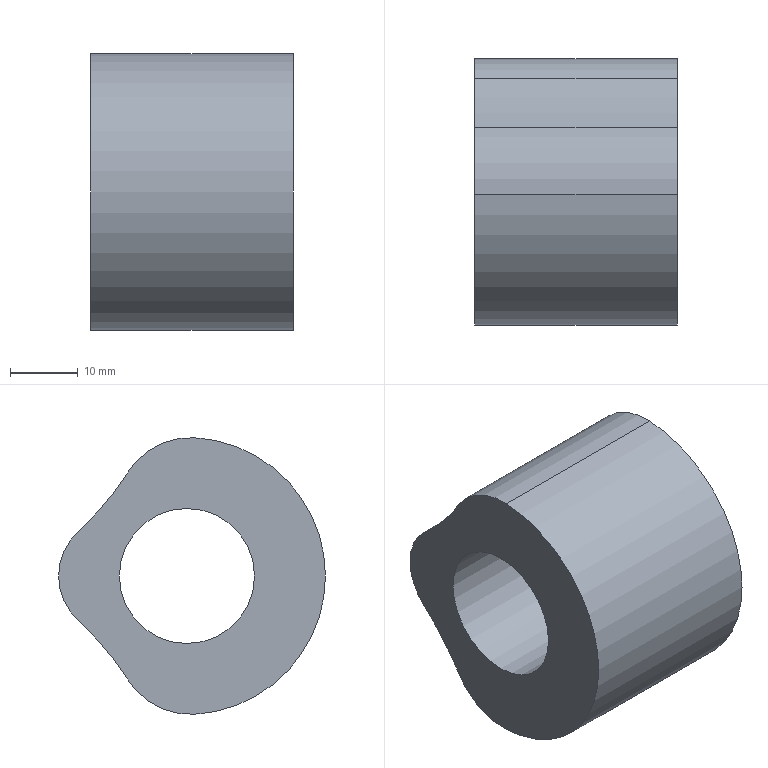Part | STEP file | cuozhitulun | 1 solid | 9 faces | box 30 x 39.5 x 40.969 mm | volume 25744 mm3 | cylinder 7 | plane 2 | commonest cylinder face diameters 22 x2 76 x2 18 x1 20 x1 41 x1
STEP:
#1=CARTESIAN_POINT('',(0.,0.,0.));
#2=DIRECTION('',(0.,0.,1.));
#3=DIRECTION('',(1.,0.,0.));
#4=AXIS2_PLACEMENT_3D('',#1,#2,#3);
#5=CARTESIAN_POINT('',(15.,8.833,-15.245));
#6=VERTEX_POINT('',#5);
#7=CARTESIAN_POINT('',(15.,15.975,-6.73));
#8=VERTEX_POINT('',#7);
#9=CARTESIAN_POINT('',(15.,41.205,-35.146));
#10=DIRECTION('',(-1.,0.,0.));
#11=DIRECTION('',(0.,0.,-1.));
#12=AXIS2_PLACEMENT_3D('',#9,#10,#11);
#13=CIRCLE('',#12,38.);
#14=CARTESIAN_POINT('',(15.,20.333,-22.315));
#15=DIRECTION('',(1.,0.,0.));
#16=DIRECTION('',(0.,0.,-1.));
#17=AXIS2_PLACEMENT_3D('',#14,#15,#16);
#18=PLANE('',#17);
#19=CARTESIAN_POINT('',(50.831,20.872));
#20=CARTESIAN_POINT('',(50.831,-44.946));
#21=CARTESIAN_POINT('',(-6.169,-12.037));
#22=CARTESIAN_POINT('',(-63.169,20.872));
#23=CARTESIAN_POINT('',(-6.169,53.781));
#24=CARTESIAN_POINT('',(50.831,86.69));
#25=CARTESIAN_POINT('',(50.831,20.872));
#26=(BOUNDED_CURVE()B_SPLINE_CURVE(2,(#19,#20,#21,#22,#23,#24,#25),.UNSPECIFIED.,.T.,.F.)B_SPLINE_CURVE_WITH_KNOTS((1,2,2,2,2,1),(-2.094,0.,2.094,4.189,6.283,8.378),.UNSPECIFIED.)CURVE()GEOMETRIC_REPRESENTATION_ITEM()RATIONAL_B_SPLINE_CURVE((1.,0.5,1.,0.5,1.,0.5,1.))REPRESENTATION_ITEM(''));
#27=(GEOMETRIC_REPRESENTATION_CONTEXT(2)PARAMETRIC_REPRESENTATION_CONTEXT()REPRESENTATION_CONTEXT('',''));
#28=DEFINITIONAL_REPRESENTATION('',(#26),#27);
#29=PCURVE('',#18,#28);
#30=CARTESIAN_POINT('',(15.,41.205,-35.146));
#31=DIRECTION('',(-1.,0.,0.));
#32=DIRECTION('',(0.,0.,1.));
#33=AXIS2_PLACEMENT_3D('',#30,#31,#32);
#34=CYLINDRICAL_SURFACE('',#33,38.);
#35=CARTESIAN_POINT('',(3.142,0.));
#36=DIRECTION('',(1.,0.));
#37=VECTOR('',#36,1.);
#38=LINE('',#35,#37);
#39=(GEOMETRIC_REPRESENTATION_CONTEXT(2)PARAMETRIC_REPRESENTATION_CONTEXT()REPRESENTATION_CONTEXT('',''));
#40=DEFINITIONAL_REPRESENTATION('',(#38),#39);
#41=PCURVE('',#34,#40);
#42=SURFACE_CURVE('',#13,(#29,#41),.PCURVE_S1.);
#43=EDGE_CURVE('',#6,#8,#42,.T.);
#44=ORIENTED_EDGE('',*,*,#43,.T.);
#45=CARTESIAN_POINT('',(15.,15.975,6.73));
#46=VERTEX_POINT('',#45);
#47=CARTESIAN_POINT('',(15.,10.,0.));
#48=DIRECTION('',(1.,0.,0.));
#49=DIRECTION('',(0.,0.,-1.));
#50=AXIS2_PLACEMENT_3D('',#47,#48,#49);
#51=CIRCLE('',#50,9.);
#52=CARTESIAN_POINT('',(-22.315,-10.333));
#53=DIRECTION('',(1.,0.));
#54=AXIS2_PLACEMENT_2D('',#52,#53);
#55=CIRCLE('',#54,9.);
#56=(GEOMETRIC_REPRESENTATION_CONTEXT(2)PARAMETRIC_REPRESENTATION_CONTEXT()REPRESENTATION_CONTEXT('',''));
#57=DEFINITIONAL_REPRESENTATION('',(#55),#56);
#58=PCURVE('',#18,#57);
#59=CARTESIAN_POINT('',(15.,10.,0.));
#60=DIRECTION('',(-1.,0.,0.));
#61=DIRECTION('',(0.,0.,1.));
#62=AXIS2_PLACEMENT_3D('',#59,#60,#61);
#63=CYLINDRICAL_SURFACE('',#62,9.);
#64=CARTESIAN_POINT('',(3.142,0.));
#65=DIRECTION('',(-1.,0.));
#66=VECTOR('',#65,1.);
#67=LINE('',#64,#66);
#68=(GEOMETRIC_REPRESENTATION_CONTEXT(2)PARAMETRIC_REPRESENTATION_CONTEXT()REPRESENTATION_CONTEXT('',''));
#69=DEFINITIONAL_REPRESENTATION('',(#67),#68);
#70=PCURVE('',#63,#69);
#71=SURFACE_CURVE('',#51,(#58,#70),.PCURVE_S1.);
#72=EDGE_CURVE('',#8,#46,#71,.T.);
#73=ORIENTED_EDGE('',*,*,#72,.T.);
#74=CARTESIAN_POINT('',(15.,8.833,15.245));
#75=VERTEX_POINT('',#74);
#76=CARTESIAN_POINT('',(15.,41.205,35.146));
#77=DIRECTION('',(-1.,0.,0.));
#78=DIRECTION('',(0.,0.,1.));
#79=AXIS2_PLACEMENT_3D('',#76,#77,#78);
#80=CIRCLE('',#79,38.);
#81=CARTESIAN_POINT('',(-95.461,20.872));
#82=CARTESIAN_POINT('',(-95.461,86.69));
#83=CARTESIAN_POINT('',(-38.461,53.781));
#84=CARTESIAN_POINT('',(18.539,20.872));
#85=CARTESIAN_POINT('',(-38.461,-12.037));
#86=CARTESIAN_POINT('',(-95.461,-44.946));
#87=CARTESIAN_POINT('',(-95.461,20.872));
#88=(BOUNDED_CURVE()B_SPLINE_CURVE(2,(#81,#82,#83,#84,#85,#86,#87),.UNSPECIFIED.,.T.,.F.)B_SPLINE_CURVE_WITH_KNOTS((1,2,2,2,2,1),(-2.094,0.,2.094,4.189,6.283,8.378),.UNSPECIFIED.)CURVE()GEOMETRIC_REPRESENTATION_ITEM()RATIONAL_B_SPLINE_CURVE((1.,0.5,1.,0.5,1.,0.5,1.))REPRESENTATION_ITEM(''));
#89=(GEOMETRIC_REPRESENTATION_CONTEXT(2)PARAMETRIC_REPRESENTATION_CONTEXT()REPRESENTATION_CONTEXT('',''));
#90=DEFINITIONAL_REPRESENTATION('',(#88),#89);
#91=PCURVE('',#18,#90);
#92=CARTESIAN_POINT('',(15.,41.205,35.146));
#93=DIRECTION('',(-1.,0.,0.));
#94=DIRECTION('',(0.,0.,1.));
#95=AXIS2_PLACEMENT_3D('',#92,#93,#94);
#96=CYLINDRICAL_SURFACE('',#95,38.);
#97=CARTESIAN_POINT('',(0.,0.));
#98=DIRECTION('',(1.,0.));
#99=VECTOR('',#98,1.);
#100=LINE('',#97,#99);
#101=(GEOMETRIC_REPRESENTATION_CONTEXT(2)PARAMETRIC_REPRESENTATION_CONTEXT()REPRESENTATION_CONTEXT('',''));
#102=DEFINITIONAL_REPRESENTATION('',(#100),#101);
#103=PCURVE('',#96,#102);
#104=SURFACE_CURVE('',#80,(#91,#103),.PCURVE_S1.);
#105=EDGE_CURVE('',#46,#75,#104,.T.);
#106=ORIENTED_EDGE('',*,*,#105,.T.);
#107=CARTESIAN_POINT('',(15.,-1.161,20.467));
#108=VERTEX_POINT('',#107);
#109=CARTESIAN_POINT('',(15.,-0.5382,9.485));
#110=DIRECTION('',(1.,0.,0.));
#111=DIRECTION('',(0.,0.,1.));
#112=AXIS2_PLACEMENT_3D('',#109,#110,#111);
#113=CIRCLE('',#112,11.);
#114=CARTESIAN_POINT('',(-31.8,-20.872));
#115=DIRECTION('',(-1.,0.));
#116=AXIS2_PLACEMENT_2D('',#114,#115);
#117=CIRCLE('',#116,11.);
#118=(GEOMETRIC_REPRESENTATION_CONTEXT(2)PARAMETRIC_REPRESENTATION_CONTEXT()REPRESENTATION_CONTEXT('',''));
#119=DEFINITIONAL_REPRESENTATION('',(#117),#118);
#120=PCURVE('',#18,#119);
#121=CARTESIAN_POINT('',(15.,-0.5382,9.485));
#122=DIRECTION('',(-1.,0.,0.));
#123=DIRECTION('',(0.,0.,1.));
#124=AXIS2_PLACEMENT_3D('',#121,#122,#123);
#125=CYLINDRICAL_SURFACE('',#124,11.);
#126=CARTESIAN_POINT('',(6.283,0.));
#127=DIRECTION('',(-1.,0.));
#128=VECTOR('',#127,1.);
#129=LINE('',#126,#128);
#130=(GEOMETRIC_REPRESENTATION_CONTEXT(2)PARAMETRIC_REPRESENTATION_CONTEXT()REPRESENTATION_CONTEXT('',''));
#131=DEFINITIONAL_REPRESENTATION('',(#129),#130);
#132=PCURVE('',#125,#131);
#133=SURFACE_CURVE('',#113,(#120,#132),.PCURVE_S1.);
#134=EDGE_CURVE('',#75,#108,#133,.T.);
#135=ORIENTED_EDGE('',*,*,#134,.T.);
#136=CARTESIAN_POINT('',(15.,-1.161,-20.467));
#137=VERTEX_POINT('',#136);
#138=CARTESIAN_POINT('',(15.,0.,0.));
#139=DIRECTION('',(1.,0.,0.));
#140=DIRECTION('',(0.,0.,-1.));
#141=AXIS2_PLACEMENT_3D('',#138,#139,#140);
#142=CIRCLE('',#141,20.5);
#143=CARTESIAN_POINT('',(-22.315,-20.333));
#144=DIRECTION('',(1.,0.));
#145=AXIS2_PLACEMENT_2D('',#143,#144);
#146=CIRCLE('',#145,20.5);
#147=(GEOMETRIC_REPRESENTATION_CONTEXT(2)PARAMETRIC_REPRESENTATION_CONTEXT()REPRESENTATION_CONTEXT('',''));
#148=DEFINITIONAL_REPRESENTATION('',(#146),#147);
#149=PCURVE('',#18,#148);
#150=CARTESIAN_POINT('',(15.,0.,0.));
#151=DIRECTION('',(-1.,0.,0.));
#152=DIRECTION('',(0.,0.,1.));
#153=AXIS2_PLACEMENT_3D('',#150,#151,#152);
#154=CYLINDRICAL_SURFACE('',#153,20.5);
#155=CARTESIAN_POINT('',(9.425,0.));
#156=DIRECTION('',(-1.,0.));
#157=VECTOR('',#156,1.);
#158=LINE('',#155,#157);
#159=(GEOMETRIC_REPRESENTATION_CONTEXT(2)PARAMETRIC_REPRESENTATION_CONTEXT()REPRESENTATION_CONTEXT('',''));
#160=DEFINITIONAL_REPRESENTATION('',(#158),#159);
#161=PCURVE('',#154,#160);
#162=SURFACE_CURVE('',#142,(#149,#161),.PCURVE_S1.);
#163=EDGE_CURVE('',#108,#137,#162,.T.);
#164=ORIENTED_EDGE('',*,*,#163,.T.);
#165=CARTESIAN_POINT('',(15.,-0.5382,-9.485));
#166=DIRECTION('',(1.,0.,0.));
#167=DIRECTION('',(0.,0.,-1.));
#168=AXIS2_PLACEMENT_3D('',#165,#166,#167);
#169=CIRCLE('',#168,11.);
#170=CARTESIAN_POINT('',(-12.831,-20.872));
#171=DIRECTION('',(1.,0.));
#172=AXIS2_PLACEMENT_2D('',#170,#171);
#173=CIRCLE('',#172,11.);
#174=(GEOMETRIC_REPRESENTATION_CONTEXT(2)PARAMETRIC_REPRESENTATION_CONTEXT()REPRESENTATION_CONTEXT('',''));
#175=DEFINITIONAL_REPRESENTATION('',(#173),#174);
#176=PCURVE('',#18,#175);
#177=CARTESIAN_POINT('',(15.,-0.5382,-9.485));
#178=DIRECTION('',(-1.,0.,0.));
#179=DIRECTION('',(0.,0.,1.));
#180=AXIS2_PLACEMENT_3D('',#177,#178,#179);
#181=CYLINDRICAL_SURFACE('',#180,11.);
#182=CARTESIAN_POINT('',(9.425,0.));
#183=DIRECTION('',(-1.,0.));
#184=VECTOR('',#183,1.);
#185=LINE('',#182,#184);
#186=(GEOMETRIC_REPRESENTATION_CONTEXT(2)PARAMETRIC_REPRESENTATION_CONTEXT()REPRESENTATION_CONTEXT('',''));
#187=DEFINITIONAL_REPRESENTATION('',(#185),#186);
#188=PCURVE('',#181,#187);
#189=SURFACE_CURVE('',#169,(#176,#188),.PCURVE_S1.);
#190=EDGE_CURVE('',#137,#6,#189,.T.);
#191=ORIENTED_EDGE('',*,*,#190,.T.);
#192=EDGE_LOOP('',(#44,#73,#106,#135,#164,#191));
#193=FACE_BOUND('',#192,.T.);
#194=CARTESIAN_POINT('',(15.,0.,-10.));
#195=VERTEX_POINT('',#194);
#196=CARTESIAN_POINT('',(15.,0.,0.));
#197=DIRECTION('',(1.,0.,0.));
#198=DIRECTION('',(0.,0.,-1.));
#199=AXIS2_PLACEMENT_3D('',#196,#197,#198);
#200=CIRCLE('',#199,10.);
#201=CARTESIAN_POINT('',(-22.315,-20.333));
#202=DIRECTION('',(1.,0.));
#203=AXIS2_PLACEMENT_2D('',#201,#202);
#204=CIRCLE('',#203,10.);
#205=(GEOMETRIC_REPRESENTATION_CONTEXT(2)PARAMETRIC_REPRESENTATION_CONTEXT()REPRESENTATION_CONTEXT('',''));
#206=DEFINITIONAL_REPRESENTATION('',(#204),#205);
#207=PCURVE('',#18,#206);
#208=CARTESIAN_POINT('',(15.,0.,0.));
#209=DIRECTION('',(-1.,0.,0.));
#210=DIRECTION('',(0.,0.,1.));
#211=AXIS2_PLACEMENT_3D('',#208,#209,#210);
#212=CYLINDRICAL_SURFACE('',#211,10.);
#213=CARTESIAN_POINT('',(9.425,0.));
#214=DIRECTION('',(-1.,0.));
#215=VECTOR('',#214,1.);
#216=LINE('',#213,#215);
#217=(GEOMETRIC_REPRESENTATION_CONTEXT(2)PARAMETRIC_REPRESENTATION_CONTEXT()REPRESENTATION_CONTEXT('',''));
#218=DEFINITIONAL_REPRESENTATION('',(#216),#217);
#219=PCURVE('',#212,#218);
#220=SURFACE_CURVE('',#200,(#207,#219),.PCURVE_S1.);
#221=EDGE_CURVE('',#195,#195,#220,.T.);
#222=ORIENTED_EDGE('',*,*,#221,.F.);
#223=EDGE_LOOP('',(#222));
#224=FACE_BOUND('',#223,.T.);
#225=ADVANCED_FACE('',(#193,#224),#18,.T.);
#226=CARTESIAN_POINT('',(-15.,8.833,-15.245));
#227=VERTEX_POINT('',#226);
#228=CARTESIAN_POINT('',(-15.,15.975,-6.73));
#229=VERTEX_POINT('',#228);
#230=CARTESIAN_POINT('',(-15.,41.205,-35.146));
#231=DIRECTION('',(-1.,0.,0.));
#232=DIRECTION('',(0.,0.,-1.));
#233=AXIS2_PLACEMENT_3D('',#230,#231,#232);
#234=CIRCLE('',#233,38.);
#235=CARTESIAN_POINT('',(-15.,20.333,-22.315));
#236=DIRECTION('',(1.,0.,0.));
#237=DIRECTION('',(0.,0.,-1.));
#238=AXIS2_PLACEMENT_3D('',#235,#236,#237);
#239=PLANE('',#238);
#240=CARTESIAN_POINT('',(50.831,20.872));
#241=CARTESIAN_POINT('',(50.831,-44.946));
#242=CARTESIAN_POINT('',(-6.169,-12.037));
#243=CARTESIAN_POINT('',(-63.169,20.872));
#244=CARTESIAN_POINT('',(-6.169,53.781));
#245=CARTESIAN_POINT('',(50.831,86.69));
#246=CARTESIAN_POINT('',(50.831,20.872));
#247=(BOUNDED_CURVE()B_SPLINE_CURVE(2,(#240,#241,#242,#243,#244,#245,#246),.UNSPECIFIED.,.T.,.F.)B_SPLINE_CURVE_WITH_KNOTS((1,2,2,2,2,1),(-2.094,0.,2.094,4.189,6.283,8.378),.UNSPECIFIED.)CURVE()GEOMETRIC_REPRESENTATION_ITEM()RATIONAL_B_SPLINE_CURVE((1.,0.5,1.,0.5,1.,0.5,1.))REPRESENTATION_ITEM(''));
#248=(GEOMETRIC_REPRESENTATION_CONTEXT(2)PARAMETRIC_REPRESENTATION_CONTEXT()REPRESENTATION_CONTEXT('',''));
#249=DEFINITIONAL_REPRESENTATION('',(#247),#248);
#250=PCURVE('',#239,#249);
#251=CARTESIAN_POINT('',(3.142,30.));
#252=DIRECTION('',(1.,0.));
#253=VECTOR('',#252,1.);
#254=LINE('',#251,#253);
#255=(GEOMETRIC_REPRESENTATION_CONTEXT(2)PARAMETRIC_REPRESENTATION_CONTEXT()REPRESENTATION_CONTEXT('',''));
#256=DEFINITIONAL_REPRESENTATION('',(#254),#255);
#257=PCURVE('',#34,#256);
#258=SURFACE_CURVE('',#234,(#250,#257),.PCURVE_S1.);
#259=EDGE_CURVE('',#227,#229,#258,.T.);
#260=ORIENTED_EDGE('',*,*,#259,.F.);
#261=CARTESIAN_POINT('',(-15.,-1.161,-20.467));
#262=VERTEX_POINT('',#261);
#263=CARTESIAN_POINT('',(-15.,-0.5382,-9.485));
#264=DIRECTION('',(1.,0.,0.));
#265=DIRECTION('',(0.,0.,-1.));
#266=AXIS2_PLACEMENT_3D('',#263,#264,#265);
#267=CIRCLE('',#266,11.);
#268=CARTESIAN_POINT('',(-12.831,-20.872));
#269=DIRECTION('',(1.,0.));
#270=AXIS2_PLACEMENT_2D('',#268,#269);
#271=CIRCLE('',#270,11.);
#272=(GEOMETRIC_REPRESENTATION_CONTEXT(2)PARAMETRIC_REPRESENTATION_CONTEXT()REPRESENTATION_CONTEXT('',''));
#273=DEFINITIONAL_REPRESENTATION('',(#271),#272);
#274=PCURVE('',#239,#273);
#275=CARTESIAN_POINT('',(9.425,30.));
#276=DIRECTION('',(-1.,0.));
#277=VECTOR('',#276,1.);
#278=LINE('',#275,#277);
#279=(GEOMETRIC_REPRESENTATION_CONTEXT(2)PARAMETRIC_REPRESENTATION_CONTEXT()REPRESENTATION_CONTEXT('',''));
#280=DEFINITIONAL_REPRESENTATION('',(#278),#279);
#281=PCURVE('',#181,#280);
#282=SURFACE_CURVE('',#267,(#274,#281),.PCURVE_S1.);
#283=EDGE_CURVE('',#262,#227,#282,.T.);
#284=ORIENTED_EDGE('',*,*,#283,.F.);
#285=CARTESIAN_POINT('',(-15.,-1.161,20.467));
#286=VERTEX_POINT('',#285);
#287=CARTESIAN_POINT('',(-15.,0.,0.));
#288=DIRECTION('',(1.,0.,0.));
#289=DIRECTION('',(0.,0.,-1.));
#290=AXIS2_PLACEMENT_3D('',#287,#288,#289);
#291=CIRCLE('',#290,20.5);
#292=CARTESIAN_POINT('',(-22.315,-20.333));
#293=DIRECTION('',(1.,0.));
#294=AXIS2_PLACEMENT_2D('',#292,#293);
#295=CIRCLE('',#294,20.5);
#296=(GEOMETRIC_REPRESENTATION_CONTEXT(2)PARAMETRIC_REPRESENTATION_CONTEXT()REPRESENTATION_CONTEXT('',''));
#297=DEFINITIONAL_REPRESENTATION('',(#295),#296);
#298=PCURVE('',#239,#297);
#299=CARTESIAN_POINT('',(9.425,30.));
#300=DIRECTION('',(-1.,0.));
#301=VECTOR('',#300,1.);
#302=LINE('',#299,#301);
#303=(GEOMETRIC_REPRESENTATION_CONTEXT(2)PARAMETRIC_REPRESENTATION_CONTEXT()REPRESENTATION_CONTEXT('',''));
#304=DEFINITIONAL_REPRESENTATION('',(#302),#303);
#305=PCURVE('',#154,#304);
#306=SURFACE_CURVE('',#291,(#298,#305),.PCURVE_S1.);
#307=EDGE_CURVE('',#286,#262,#306,.T.);
#308=ORIENTED_EDGE('',*,*,#307,.F.);
#309=CARTESIAN_POINT('',(-15.,8.833,15.245));
#310=VERTEX_POINT('',#309);
#311=CARTESIAN_POINT('',(-15.,-0.5382,9.485));
#312=DIRECTION('',(1.,0.,0.));
#313=DIRECTION('',(0.,0.,1.));
#314=AXIS2_PLACEMENT_3D('',#311,#312,#313);
#315=CIRCLE('',#314,11.);
#316=CARTESIAN_POINT('',(-31.8,-20.872));
#317=DIRECTION('',(-1.,0.));
#318=AXIS2_PLACEMENT_2D('',#316,#317);
#319=CIRCLE('',#318,11.);
#320=(GEOMETRIC_REPRESENTATION_CONTEXT(2)PARAMETRIC_REPRESENTATION_CONTEXT()REPRESENTATION_CONTEXT('',''));
#321=DEFINITIONAL_REPRESENTATION('',(#319),#320);
#322=PCURVE('',#239,#321);
#323=CARTESIAN_POINT('',(6.283,30.));
#324=DIRECTION('',(-1.,0.));
#325=VECTOR('',#324,1.);
#326=LINE('',#323,#325);
#327=(GEOMETRIC_REPRESENTATION_CONTEXT(2)PARAMETRIC_REPRESENTATION_CONTEXT()REPRESENTATION_CONTEXT('',''));
#328=DEFINITIONAL_REPRESENTATION('',(#326),#327);
#329=PCURVE('',#125,#328);
#330=SURFACE_CURVE('',#315,(#322,#329),.PCURVE_S1.);
#331=EDGE_CURVE('',#310,#286,#330,.T.);
#332=ORIENTED_EDGE('',*,*,#331,.F.);
#333=CARTESIAN_POINT('',(-15.,15.975,6.73));
#334=VERTEX_POINT('',#333);
#335=CARTESIAN_POINT('',(-15.,41.205,35.146));
#336=DIRECTION('',(-1.,0.,0.));
#337=DIRECTION('',(0.,0.,1.));
#338=AXIS2_PLACEMENT_3D('',#335,#336,#337);
#339=CIRCLE('',#338,38.);
#340=CARTESIAN_POINT('',(-95.461,20.872));
#341=CARTESIAN_POINT('',(-95.461,86.69));
#342=CARTESIAN_POINT('',(-38.461,53.781));
#343=CARTESIAN_POINT('',(18.539,20.872));
#344=CARTESIAN_POINT('',(-38.461,-12.037));
#345=CARTESIAN_POINT('',(-95.461,-44.946));
#346=CARTESIAN_POINT('',(-95.461,20.872));
#347=(BOUNDED_CURVE()B_SPLINE_CURVE(2,(#340,#341,#342,#343,#344,#345,#346),.UNSPECIFIED.,.T.,.F.)B_SPLINE_CURVE_WITH_KNOTS((1,2,2,2,2,1),(-2.094,0.,2.094,4.189,6.283,8.378),.UNSPECIFIED.)CURVE()GEOMETRIC_REPRESENTATION_ITEM()RATIONAL_B_SPLINE_CURVE((1.,0.5,1.,0.5,1.,0.5,1.))REPRESENTATION_ITEM(''));
#348=(GEOMETRIC_REPRESENTATION_CONTEXT(2)PARAMETRIC_REPRESENTATION_CONTEXT()REPRESENTATION_CONTEXT('',''));
#349=DEFINITIONAL_REPRESENTATION('',(#347),#348);
#350=PCURVE('',#239,#349);
#351=CARTESIAN_POINT('',(0.,30.));
#352=DIRECTION('',(1.,0.));
#353=VECTOR('',#352,1.);
#354=LINE('',#351,#353);
#355=(GEOMETRIC_REPRESENTATION_CONTEXT(2)PARAMETRIC_REPRESENTATION_CONTEXT()REPRESENTATION_CONTEXT('',''));
#356=DEFINITIONAL_REPRESENTATION('',(#354),#355);
#357=PCURVE('',#96,#356);
#358=SURFACE_CURVE('',#339,(#350,#357),.PCURVE_S1.);
#359=EDGE_CURVE('',#334,#310,#358,.T.);
#360=ORIENTED_EDGE('',*,*,#359,.F.);
#361=CARTESIAN_POINT('',(-15.,10.,0.));
#362=DIRECTION('',(1.,0.,0.));
#363=DIRECTION('',(0.,0.,-1.));
#364=AXIS2_PLACEMENT_3D('',#361,#362,#363);
#365=CIRCLE('',#364,9.);
#366=CARTESIAN_POINT('',(-22.315,-10.333));
#367=DIRECTION('',(1.,0.));
#368=AXIS2_PLACEMENT_2D('',#366,#367);
#369=CIRCLE('',#368,9.);
#370=(GEOMETRIC_REPRESENTATION_CONTEXT(2)PARAMETRIC_REPRESENTATION_CONTEXT()REPRESENTATION_CONTEXT('',''));
#371=DEFINITIONAL_REPRESENTATION('',(#369),#370);
#372=PCURVE('',#239,#371);
#373=CARTESIAN_POINT('',(3.142,30.));
#374=DIRECTION('',(-1.,0.));
#375=VECTOR('',#374,1.);
#376=LINE('',#373,#375);
#377=(GEOMETRIC_REPRESENTATION_CONTEXT(2)PARAMETRIC_REPRESENTATION_CONTEXT()REPRESENTATION_CONTEXT('',''));
#378=DEFINITIONAL_REPRESENTATION('',(#376),#377);
#379=PCURVE('',#63,#378);
#380=SURFACE_CURVE('',#365,(#372,#379),.PCURVE_S1.);
#381=EDGE_CURVE('',#229,#334,#380,.T.);
#382=ORIENTED_EDGE('',*,*,#381,.F.);
#383=EDGE_LOOP('',(#260,#284,#308,#332,#360,#382));
#384=FACE_BOUND('',#383,.T.);
#385=CARTESIAN_POINT('',(-15.,0.,-10.));
#386=VERTEX_POINT('',#385);
#387=CARTESIAN_POINT('',(-15.,0.,0.));
#388=DIRECTION('',(1.,0.,0.));
#389=DIRECTION('',(0.,0.,-1.));
#390=AXIS2_PLACEMENT_3D('',#387,#388,#389);
#391=CIRCLE('',#390,10.);
#392=CARTESIAN_POINT('',(-22.315,-20.333));
#393=DIRECTION('',(1.,0.));
#394=AXIS2_PLACEMENT_2D('',#392,#393);
#395=CIRCLE('',#394,10.);
#396=(GEOMETRIC_REPRESENTATION_CONTEXT(2)PARAMETRIC_REPRESENTATION_CONTEXT()REPRESENTATION_CONTEXT('',''));
#397=DEFINITIONAL_REPRESENTATION('',(#395),#396);
#398=PCURVE('',#239,#397);
#399=CARTESIAN_POINT('',(9.425,30.));
#400=DIRECTION('',(-1.,0.));
#401=VECTOR('',#400,1.);
#402=LINE('',#399,#401);
#403=(GEOMETRIC_REPRESENTATION_CONTEXT(2)PARAMETRIC_REPRESENTATION_CONTEXT()REPRESENTATION_CONTEXT('',''));
#404=DEFINITIONAL_REPRESENTATION('',(#402),#403);
#405=PCURVE('',#212,#404);
#406=SURFACE_CURVE('',#391,(#398,#405),.PCURVE_S1.);
#407=EDGE_CURVE('',#386,#386,#406,.T.);
#408=ORIENTED_EDGE('',*,*,#407,.T.);
#409=EDGE_LOOP('',(#408));
#410=FACE_BOUND('',#409,.T.);
#411=ADVANCED_FACE('',(#384,#410),#239,.F.);
#412=CARTESIAN_POINT('',(15.,8.833,-15.245));
#413=DIRECTION('',(-1.,0.,0.));
#414=VECTOR('',#413,1.);
#415=LINE('',#412,#414);
#416=CARTESIAN_POINT('',(5.264,0.));
#417=DIRECTION('',(0.,1.));
#418=VECTOR('',#417,1.);
#419=LINE('',#416,#418);
#420=(GEOMETRIC_REPRESENTATION_CONTEXT(2)PARAMETRIC_REPRESENTATION_CONTEXT()REPRESENTATION_CONTEXT('',''));
#421=DEFINITIONAL_REPRESENTATION('',(#419),#420);
#422=PCURVE('',#34,#421);
#423=CARTESIAN_POINT('',(2.122,0.));
#424=DIRECTION('',(0.,1.));
#425=VECTOR('',#424,1.);
#426=LINE('',#423,#425);
#427=(GEOMETRIC_REPRESENTATION_CONTEXT(2)PARAMETRIC_REPRESENTATION_CONTEXT()REPRESENTATION_CONTEXT('',''));
#428=DEFINITIONAL_REPRESENTATION('',(#426),#427);
#429=PCURVE('',#181,#428);
#430=SURFACE_CURVE('',#415,(#422,#429),.PCURVE_S1.);
#431=EDGE_CURVE('',#6,#227,#430,.T.);
#432=ORIENTED_EDGE('',*,*,#431,.F.);
#433=ORIENTED_EDGE('',*,*,#43,.T.);
#434=CARTESIAN_POINT('',(15.,15.975,-6.73));
#435=DIRECTION('',(-1.,0.,0.));
#436=VECTOR('',#435,1.);
#437=LINE('',#434,#436);
#438=CARTESIAN_POINT('',(5.557,0.));
#439=DIRECTION('',(0.,1.));
#440=VECTOR('',#439,1.);
#441=LINE('',#438,#440);
#442=(GEOMETRIC_REPRESENTATION_CONTEXT(2)PARAMETRIC_REPRESENTATION_CONTEXT()REPRESENTATION_CONTEXT('',''));
#443=DEFINITIONAL_REPRESENTATION('',(#441),#442);
#444=PCURVE('',#34,#443);
#445=CARTESIAN_POINT('',(2.416,0.));
#446=DIRECTION('',(0.,1.));
#447=VECTOR('',#446,1.);
#448=LINE('',#445,#447);
#449=(GEOMETRIC_REPRESENTATION_CONTEXT(2)PARAMETRIC_REPRESENTATION_CONTEXT()REPRESENTATION_CONTEXT('',''));
#450=DEFINITIONAL_REPRESENTATION('',(#448),#449);
#451=PCURVE('',#63,#450);
#452=SURFACE_CURVE('',#437,(#444,#451),.PCURVE_S1.);
#453=EDGE_CURVE('',#8,#229,#452,.T.);
#454=ORIENTED_EDGE('',*,*,#453,.T.);
#455=ORIENTED_EDGE('',*,*,#259,.F.);
#456=EDGE_LOOP('',(#432,#433,#454,#455));
#457=FACE_BOUND('',#456,.F.);
#458=ADVANCED_FACE('',(#457),#34,.F.);
#459=ORIENTED_EDGE('',*,*,#381,.T.);
#460=CARTESIAN_POINT('',(15.,15.975,6.73));
#461=DIRECTION('',(-1.,0.,0.));
#462=VECTOR('',#461,1.);
#463=LINE('',#460,#462);
#464=CARTESIAN_POINT('',(0.7261,0.));
#465=DIRECTION('',(0.,1.));
#466=VECTOR('',#465,1.);
#467=LINE('',#464,#466);
#468=(GEOMETRIC_REPRESENTATION_CONTEXT(2)PARAMETRIC_REPRESENTATION_CONTEXT()REPRESENTATION_CONTEXT('',''));
#469=DEFINITIONAL_REPRESENTATION('',(#467),#468);
#470=PCURVE('',#63,#469);
#471=CARTESIAN_POINT('',(3.868,0.));
#472=DIRECTION('',(0.,1.));
#473=VECTOR('',#472,1.);
#474=LINE('',#471,#473);
#475=(GEOMETRIC_REPRESENTATION_CONTEXT(2)PARAMETRIC_REPRESENTATION_CONTEXT()REPRESENTATION_CONTEXT('',''));
#476=DEFINITIONAL_REPRESENTATION('',(#474),#475);
#477=PCURVE('',#96,#476);
#478=SURFACE_CURVE('',#463,(#470,#477),.PCURVE_S1.);
#479=EDGE_CURVE('',#46,#334,#478,.T.);
#480=ORIENTED_EDGE('',*,*,#479,.F.);
#481=ORIENTED_EDGE('',*,*,#72,.F.);
#482=ORIENTED_EDGE('',*,*,#453,.T.);
#483=EDGE_LOOP('',(#459,#480,#481,#482));
#484=FACE_BOUND('',#483,.T.);
#485=ADVANCED_FACE('',(#484),#63,.T.);
#486=ORIENTED_EDGE('',*,*,#479,.F.);
#487=ORIENTED_EDGE('',*,*,#105,.T.);
#488=CARTESIAN_POINT('',(15.,8.833,15.245));
#489=DIRECTION('',(-1.,0.,0.));
#490=VECTOR('',#489,1.);
#491=LINE('',#488,#490);
#492=CARTESIAN_POINT('',(4.161,0.));
#493=DIRECTION('',(0.,1.));
#494=VECTOR('',#493,1.);
#495=LINE('',#492,#494);
#496=(GEOMETRIC_REPRESENTATION_CONTEXT(2)PARAMETRIC_REPRESENTATION_CONTEXT()REPRESENTATION_CONTEXT('',''));
#497=DEFINITIONAL_REPRESENTATION('',(#495),#496);
#498=PCURVE('',#96,#497);
#499=CARTESIAN_POINT('',(1.02,0.));
#500=DIRECTION('',(0.,1.));
#501=VECTOR('',#500,1.);
#502=LINE('',#499,#501);
#503=(GEOMETRIC_REPRESENTATION_CONTEXT(2)PARAMETRIC_REPRESENTATION_CONTEXT()REPRESENTATION_CONTEXT('',''));
#504=DEFINITIONAL_REPRESENTATION('',(#502),#503);
#505=PCURVE('',#125,#504);
#506=SURFACE_CURVE('',#491,(#498,#505),.PCURVE_S1.);
#507=EDGE_CURVE('',#75,#310,#506,.T.);
#508=ORIENTED_EDGE('',*,*,#507,.T.);
#509=ORIENTED_EDGE('',*,*,#359,.F.);
#510=EDGE_LOOP('',(#486,#487,#508,#509));
#511=FACE_BOUND('',#510,.F.);
#512=ADVANCED_FACE('',(#511),#96,.F.);
#513=ORIENTED_EDGE('',*,*,#331,.T.);
#514=CARTESIAN_POINT('',(15.,-1.161,20.467));
#515=DIRECTION('',(-1.,0.,0.));
#516=VECTOR('',#515,1.);
#517=LINE('',#514,#516);
#518=CARTESIAN_POINT('',(-0.05668,0.));
#519=DIRECTION('',(0.,1.));
#520=VECTOR('',#519,1.);
#521=LINE('',#518,#520);
#522=(GEOMETRIC_REPRESENTATION_CONTEXT(2)PARAMETRIC_REPRESENTATION_CONTEXT()REPRESENTATION_CONTEXT('',''));
#523=DEFINITIONAL_REPRESENTATION('',(#521),#522);
#524=PCURVE('',#125,#523);
#525=CARTESIAN_POINT('',(6.227,0.));
#526=DIRECTION('',(0.,1.));
#527=VECTOR('',#526,1.);
#528=LINE('',#525,#527);
#529=(GEOMETRIC_REPRESENTATION_CONTEXT(2)PARAMETRIC_REPRESENTATION_CONTEXT()REPRESENTATION_CONTEXT('',''));
#530=DEFINITIONAL_REPRESENTATION('',(#528),#529);
#531=PCURVE('',#154,#530);
#532=SURFACE_CURVE('',#517,(#524,#531),.PCURVE_S1.);
#533=EDGE_CURVE('',#108,#286,#532,.T.);
#534=ORIENTED_EDGE('',*,*,#533,.F.);
#535=ORIENTED_EDGE('',*,*,#134,.F.);
#536=ORIENTED_EDGE('',*,*,#507,.T.);
#537=EDGE_LOOP('',(#513,#534,#535,#536));
#538=FACE_BOUND('',#537,.T.);
#539=ADVANCED_FACE('',(#538),#125,.T.);
#540=ORIENTED_EDGE('',*,*,#307,.T.);
#541=CARTESIAN_POINT('',(15.,-1.161,-20.467));
#542=DIRECTION('',(-1.,0.,0.));
#543=VECTOR('',#542,1.);
#544=LINE('',#541,#543);
#545=CARTESIAN_POINT('',(3.198,0.));
#546=DIRECTION('',(0.,1.));
#547=VECTOR('',#546,1.);
#548=LINE('',#545,#547);
#549=(GEOMETRIC_REPRESENTATION_CONTEXT(2)PARAMETRIC_REPRESENTATION_CONTEXT()REPRESENTATION_CONTEXT('',''));
#550=DEFINITIONAL_REPRESENTATION('',(#548),#549);
#551=PCURVE('',#154,#550);
#552=CARTESIAN_POINT('',(3.198,0.));
#553=DIRECTION('',(0.,1.));
#554=VECTOR('',#553,1.);
#555=LINE('',#552,#554);
#556=(GEOMETRIC_REPRESENTATION_CONTEXT(2)PARAMETRIC_REPRESENTATION_CONTEXT()REPRESENTATION_CONTEXT('',''));
#557=DEFINITIONAL_REPRESENTATION('',(#555),#556);
#558=PCURVE('',#181,#557);
#559=SURFACE_CURVE('',#544,(#551,#558),.PCURVE_S1.);
#560=EDGE_CURVE('',#137,#262,#559,.T.);
#561=ORIENTED_EDGE('',*,*,#560,.F.);
#562=ORIENTED_EDGE('',*,*,#163,.F.);
#563=ORIENTED_EDGE('',*,*,#533,.T.);
#564=EDGE_LOOP('',(#540,#561,#562,#563));
#565=FACE_BOUND('',#564,.T.);
#566=ADVANCED_FACE('',(#565),#154,.T.);
#567=ORIENTED_EDGE('',*,*,#283,.T.);
#568=ORIENTED_EDGE('',*,*,#431,.F.);
#569=ORIENTED_EDGE('',*,*,#190,.F.);
#570=ORIENTED_EDGE('',*,*,#560,.T.);
#571=EDGE_LOOP('',(#567,#568,#569,#570));
#572=FACE_BOUND('',#571,.T.);
#573=ADVANCED_FACE('',(#572),#181,.T.);
#574=ORIENTED_EDGE('',*,*,#221,.F.);
#575=CARTESIAN_POINT('',(15.,0.,-10.));
#576=CARTESIAN_POINT('',(-15.,0.,-10.));
#577=B_SPLINE_CURVE_WITH_KNOTS('',1,(#575,#576),.UNSPECIFIED.,.F.,.F.,(2,2),(0.,30.),.PIECEWISE_BEZIER_KNOTS.);
#578=CARTESIAN_POINT('',(9.425,0.));
#579=DIRECTION('',(0.,1.));
#580=VECTOR('',#579,1.);
#581=LINE('',#578,#580);
#582=(GEOMETRIC_REPRESENTATION_CONTEXT(2)PARAMETRIC_REPRESENTATION_CONTEXT()REPRESENTATION_CONTEXT('',''));
#583=DEFINITIONAL_REPRESENTATION('',(#581),#582);
#584=PCURVE('',#212,#583);
#585=CARTESIAN_POINT('',(3.142,0.));
#586=DIRECTION('',(0.,1.));
#587=VECTOR('',#586,1.);
#588=LINE('',#585,#587);
#589=(GEOMETRIC_REPRESENTATION_CONTEXT(2)PARAMETRIC_REPRESENTATION_CONTEXT()REPRESENTATION_CONTEXT('',''));
#590=DEFINITIONAL_REPRESENTATION('',(#588),#589);
#591=PCURVE('',#212,#590);
#592=SEAM_CURVE('',#577,(#584,#591),.PCURVE_S1.);
#593=EDGE_CURVE('',#195,#386,#592,.T.);
#594=ORIENTED_EDGE('',*,*,#593,.T.);
#595=ORIENTED_EDGE('',*,*,#407,.T.);
#596=ORIENTED_EDGE('',*,*,#593,.F.);
#597=EDGE_LOOP('',(#574,#594,#595,#596));
#598=FACE_BOUND('',#597,.F.);
#599=ADVANCED_FACE('',(#598),#212,.F.);
#600=CLOSED_SHELL('',(#225,#411,#458,#485,#512,#539,#566,#573,#599));
#601=MANIFOLD_SOLID_BREP('',#600);
#602=(LENGTH_UNIT()NAMED_UNIT(*)SI_UNIT(.MILLI.,.METRE.));
#603=UNCERTAINTY_MEASURE_WITH_UNIT(LENGTH_MEASURE(0.000001),#602,'','');
#604=(NAMED_UNIT(*)PLANE_ANGLE_UNIT()SI_UNIT($,.RADIAN.));
#605=(NAMED_UNIT(*)SI_UNIT($,.STERADIAN.)SOLID_ANGLE_UNIT());
#606=(GEOMETRIC_REPRESENTATION_CONTEXT(3)GLOBAL_UNCERTAINTY_ASSIGNED_CONTEXT((#603))GLOBAL_UNIT_ASSIGNED_CONTEXT((#602,#604,#605))REPRESENTATION_CONTEXT('',''));
#607=ADVANCED_BREP_SHAPE_REPRESENTATION('',(#4,#601),#606);